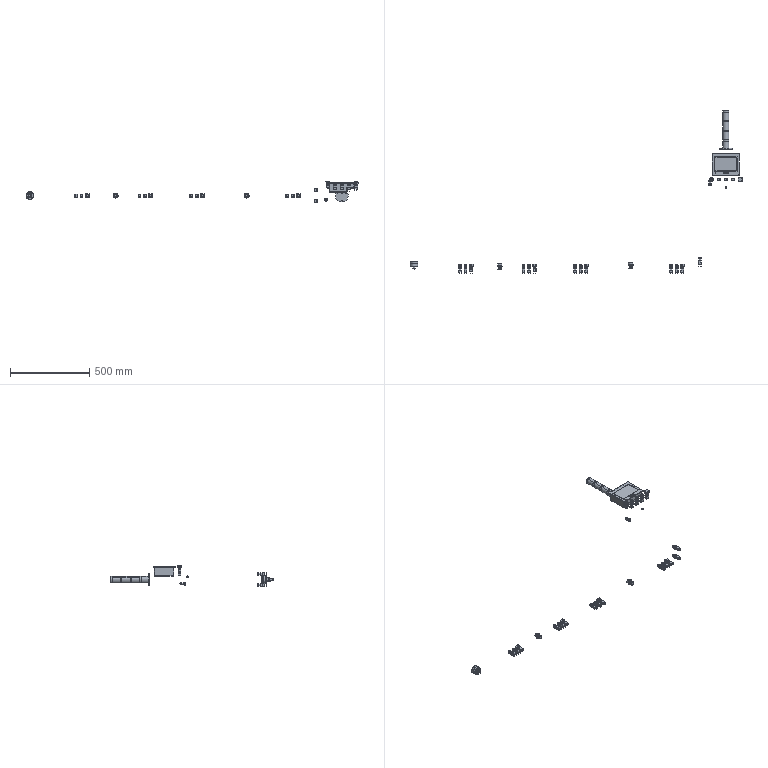Part | NX | 37 solids | 2589 faces | box 2092 x 1029 x 133.2 mm | volume 1515555 mm3 | plane 1950 | cylinder 542 | torus 46 | cone 36 | sphere 11 | spline 4 | commonest cylinder face diameters 1 x96 21 x72 15.6 x64 18 x41 17.9 x38 1.9 x20